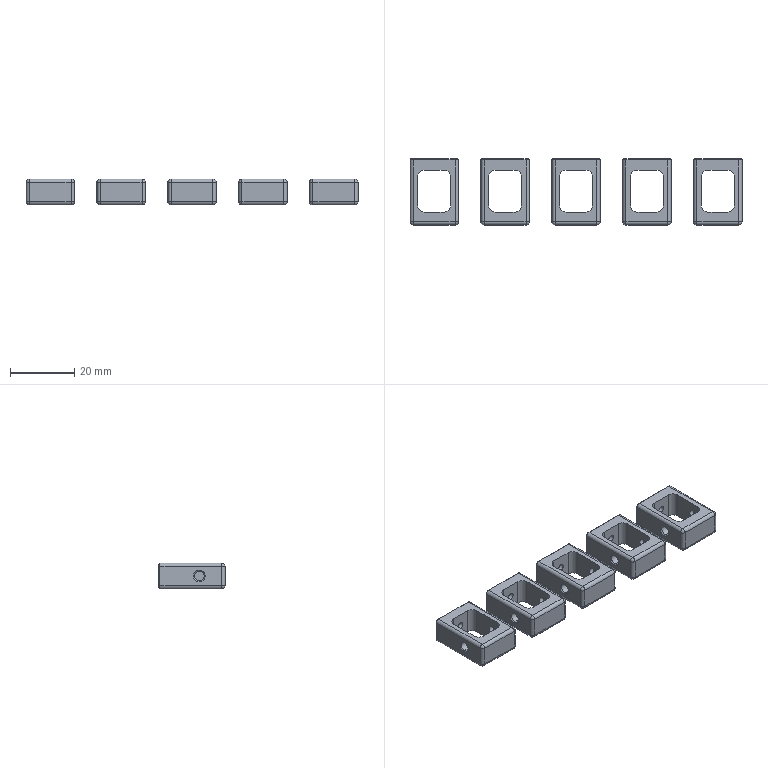NC program | NX | posted with a generic post | part box 103 x 20.5 x 8 mm
Lines 4727 to 5798 of 9732:
(ZLEVEL_PROFILE_COPY_1 , TOOL : D4)
N9440 T11 M6
N9442 G54
N9444 G17 G0 G90 X45.472 Y-3.85 S9950 M3
N9446 G43 Z30. H11
N9448 Z0.6
N9450 G94 G1 Z-0.4 F1000.
N9452 X45.587 Y-4.05
N9454 G3 X45.934 Y-4.25 R0.4
N9456 G1 X47.1 F1600.
N9458 Y-3.095
N9460 G3 X46.9 Y-2.749 R0.4
N9462 G1 X46.7 Y-2.634
N9464 Z0.6
N9466 G0 X45.472 Y-3.85 Z0.2
N9468 G1 Z-0.8 F1000.
N9470 X45.587 Y-4.05
N9472 G3 X45.934 Y-4.25 R0.4
N9474 G1 X47.1 F1600.
N9476 Y-3.095
N9478 G3 X46.9 Y-2.749 R0.4
N9480 G1 X46.7 Y-2.634
N9482 Z0.2
N9484 G0 X45.472 Y-3.85 Z-0.2
N9486 G1 Z-1.2 F1000.
N9488 X45.587 Y-4.05
N9490 G3 X45.934 Y-4.25 R0.4
N9492 G1 X47.1 F1600.
N9494 Y-3.095
N9496 G3 X46.9 Y-2.749 R0.4
N9498 G1 X46.7 Y-2.634
N9500 Z-0.2
N9502 G0 X45.472 Y-3.85 Z-0.6
N9504 G1 Z-1.6 F1000.
N9506 X45.587 Y-4.05
N9508 G3 X45.934 Y-4.25 R0.4
N9510 G1 X47.1 F1600.
N9512 Y-3.095
N9514 G3 X46.9 Y-2.749 R0.4
N9516 G1 X46.7 Y-2.634
N9518 Z-0.6
N9520 G0 X45.472 Y-3.85 Z-1.
N9522 G1 Z-2. F1000.
N9524 X45.587 Y-4.05
N9526 G3 X45.934 Y-4.25 R0.4
N9528 G1 X47.1 F1600.
N9530 Y-3.095
N9532 G3 X46.9 Y-2.749 R0.4
N9534 G1 X46.7 Y-2.634
N9536 Z-1.
N9538 G0 X45.472 Y-3.85 Z-1.4
N9540 G1 Z-2.4 F1000.
N9542 X45.587 Y-4.05
N9544 G3 X45.934 Y-4.25 R0.4
N9546 G1 X47.1 F1600.
N9548 Y-3.095
N9550 G3 X46.9 Y-2.749 R0.4
N9552 G1 X46.7 Y-2.634
N9554 Z-1.4
N9556 G0 X45.472 Y-3.85 Z-1.8
N9558 G1 Z-2.8 F1000.
N9560 X45.587 Y-4.05
N9562 G3 X45.934 Y-4.25 R0.4
N9564 G1 X47.1 F1600.
N9566 Y-3.095
N9568 G3 X46.9 Y-2.749 R0.4
N9570 G1 X46.7 Y-2.634
N9572 Z-1.8
N9574 G0 X45.472 Y-3.85 Z-2.2
N9576 G1 Z-3.2 F1000.
N9578 X45.587 Y-4.05
N9580 G3 X45.934 Y-4.25 R0.4
N9582 G1 X47.1 F1600.
N9584 Y-3.095
N9586 G3 X46.9 Y-2.749 R0.4
N9588 G1 X46.7 Y-2.634
N9590 Z-2.2
N9592 G0 X45.472 Y-3.85 Z-2.6
N9594 G1 Z-3.6 F1000.
N9596 X45.587 Y-4.05
N9598 G3 X45.934 Y-4.25 R0.4
N9600 G1 X47.1 F1600.
N9602 Y-3.095
N9604 G3 X46.9 Y-2.749 R0.4
N9606 G1 X46.7 Y-2.634
N9608 Z-2.6
N9610 G0 X45.472 Y-3.85 Z-3.
N9612 G1 Z-4. F1000.
N9614 X45.587 Y-4.05
N9616 G3 X45.934 Y-4.25 R0.4
N9618 G1 X47.1 F1600.
N9620 Y-3.095
N9622 G3 X46.9 Y-2.749 R0.4
N9624 G1 X46.7 Y-2.634
N9626 Z-3.
N9628 G0 X45.472 Y-3.85 Z-3.4
N9630 G1 Z-4.4 F1000.
N9632 X45.587 Y-4.05
N9634 G3 X45.934 Y-4.25 R0.4
N9636 G1 X47.1 F1600.
N9638 Y-3.095
N9640 G3 X46.9 Y-2.749 R0.4
N9642 G1 X46.7 Y-2.634
N9644 Z-3.4
N9646 G0 X45.472 Y-3.85 Z-3.8
N9648 G1 Z-4.8 F1000.
N9650 X45.587 Y-4.05
N9652 G3 X45.934 Y-4.25 R0.4
N9654 G1 X47.1 F1600.
N9656 Y-3.095
N9658 G3 X46.9 Y-2.749 R0.4
N9660 G1 X46.7 Y-2.634
N9662 Z-3.8
N9664 G0 X45.472 Y-3.85 Z-4.2
N9666 G1 Z-5.2 F1000.
N9668 X45.587 Y-4.05
N9670 G3 X45.934 Y-4.25 R0.4
N9672 G1 X47.1 F1600.
N9674 Y-3.095
N9676 G3 X46.9 Y-2.749 R0.4
N9678 G1 X46.7 Y-2.634
N9680 Z-4.2
N9682 G0 X45.472 Y-3.85 Z-4.6
N9684 G1 Z-5.6 F1000.
N9686 X45.587 Y-4.05
N9688 G3 X45.934 Y-4.25 R0.4
N9690 G1 X47.1 F1600.
N9692 Y-3.095
N9694 G3 X46.9 Y-2.749 R0.4
N9696 G1 X46.7 Y-2.634
N9698 Z-4.6
N9700 G0 X45.472 Y-3.85 Z-5.
N9702 G1 Z-6. F1000.
N9704 X45.587 Y-4.05
N9706 G3 X45.934 Y-4.25 R0.4
N9708 G1 X47.1 F1600.
N9710 Y-3.095
N9712 G3 X46.9 Y-2.749 R0.4
N9714 G1 X46.7 Y-2.634
N9716 Z-5.
N9718 G0 X45.472 Y-3.85 Z-5.4
N9720 G1 Z-6.4 F1000.
N9722 X45.587 Y-4.05
N9724 G3 X45.934 Y-4.25 R0.4
N9726 G1 X47.1 F1600.
N9728 Y-3.095
N9730 G3 X46.9 Y-2.749 R0.4
N9732 G1 X46.7 Y-2.634
N9734 Z-5.4
N9736 G0 X45.472 Y-3.85 Z-5.8
N9738 G1 Z-6.8 F1000.
N9740 X45.587 Y-4.05
N9742 G3 X45.934 Y-4.25 R0.4
N9744 G1 X47.1 F1600.
N9746 Y-3.095
N9748 G3 X46.9 Y-2.749 R0.4
N9750 G1 X46.7 Y-2.634
N9752 Z-5.8
N9754 G0 X45.472 Y-3.85 Z-6.2
N9756 G1 Z-7.2 F1000.
N9758 X45.587 Y-4.05
N9760 G3 X45.934 Y-4.25 R0.4
N9762 G1 X47.1 F1600.
N9764 Y-3.095
N9766 G3 X46.9 Y-2.749 R0.4
N9768 G1 X46.7 Y-2.634
N9770 Z-6.2
N9772 G0 X45.472 Y-3.85 Z-6.6
N9774 G1 Z-7.6 F1000.
N9776 X45.587 Y-4.05
N9778 G3 X45.934 Y-4.25 R0.4
N9780 G1 X47.1 F1600.
N9782 Y-3.095
N9784 G3 X46.9 Y-2.749 R0.4
N9786 G1 X46.7 Y-2.634
N9788 Z-6.6
N9790 G0 X45.472 Y-3.85 Z-7.
N9792 G1 Z-8. F1000.
N9794 X45.587 Y-4.05
N9796 G3 X45.934 Y-4.25 R0.4
N9798 G1 X47.1 F1600.
N9800 Y-3.095
N9802 G3 X46.9 Y-2.749 R0.4
N9804 G1 X46.7 Y-2.634
N9806 Z-7.
N9808 G0 Z30.
N9810 Y3.14
N9812 Z0.6
N9814 G1 Z-0.4 F1000.
N9816 X46.9 Y3.256
N9818 G3 X47.1 Y3.602 R0.4
N9820 G1 Y4.75 F1600.
N9822 X45.952
N9824 G3 X45.606 Y4.55 R0.4
N9826 G1 X45.49 Y4.35
N9828 Z0.6
N9830 G0 X46.7 Y3.14 Z0.2
N9832 G1 Z-0.8 F1000.
N9834 X46.9 Y3.256
N9836 G3 X47.1 Y3.602 R0.4
N9838 G1 Y4.75 F1600.
N9840 X45.952
N9842 G3 X45.606 Y4.55 R0.4
N9844 G1 X45.49 Y4.35
N9846 Z0.2
N9848 G0 X46.7 Y3.14 Z-0.2
N9850 G1 Z-1.2 F1000.
N9852 X46.9 Y3.256
N9854 G3 X47.1 Y3.602 R0.4
N9856 G1 Y4.75 F1600.
N9858 X45.952
N9860 G3 X45.606 Y4.55 R0.4
N9862 G1 X45.49 Y4.35
N9864 Z-0.2
N9866 G0 X46.7 Y3.14 Z-0.6
N9868 G1 Z-1.6 F1000.
N9870 X46.9 Y3.256
N9872 G3 X47.1 Y3.602 R0.4
N9874 G1 Y4.75 F1600.
N9876 X45.952
N9878 G3 X45.606 Y4.55 R0.4
N9880 G1 X45.49 Y4.35
N9882 Z-0.6
N9884 G0 X46.7 Y3.14 Z-1.
N9886 G1 Z-2. F1000.
N9888 X46.9 Y3.256
N9890 G3 X47.1 Y3.602 R0.4
N9892 G1 Y4.75 F1600.
N9894 X45.952
N9896 G3 X45.606 Y4.55 R0.4
N9898 G1 X45.49 Y4.35
N9900 Z-1.
N9902 G0 X46.7 Y3.14 Z-1.4
N9904 G1 Z-2.4 F1000.
N9906 X46.9 Y3.256
N9908 G3 X47.1 Y3.602 R0.4
N9910 G1 Y4.75 F1600.
N9912 X45.952
N9914 G3 X45.606 Y4.55 R0.4
N9916 G1 X45.49 Y4.35
N9918 Z-1.4
N9920 G0 X46.7 Y3.14 Z-1.8
N9922 G1 Z-2.8 F1000.
N9924 X46.9 Y3.256
N9926 G3 X47.1 Y3.602 R0.4
N9928 G1 Y4.75 F1600.
N9930 X45.952
N9932 G3 X45.606 Y4.55 R0.4
N9934 G1 X45.49 Y4.35
N9936 Z-1.8
N9938 G0 X46.7 Y3.14 Z-2.2
N9940 G1 Z-3.2 F1000.
N9942 X46.9 Y3.256
N9944 G3 X47.1 Y3.602 R0.4
N9946 G1 Y4.75 F1600.
N9948 X45.952
N9950 G3 X45.606 Y4.55 R0.4
N9952 G1 X45.49 Y4.35
N9954 Z-2.2
N9956 G0 X46.7 Y3.14 Z-2.6
N9958 G1 Z-3.6 F1000.
N9960 X46.9 Y3.256
N9962 G3 X47.1 Y3.602 R0.4
N9964 G1 Y4.75 F1600.
N9966 X45.952
N9968 G3 X45.606 Y4.55 R0.4
N9970 G1 X45.49 Y4.35
N9972 Z-2.6
N9974 G0 X46.7 Y3.14 Z-3.
N9976 G1 Z-4. F1000.
N9978 X46.9 Y3.256
N9980 G3 X47.1 Y3.602 R0.4
N9982 G1 Y4.75 F1600.
N9984 X45.952
N9986 G3 X45.606 Y4.55 R0.4
N9988 G1 X45.49 Y4.35
N9990 Z-3.
N9992 G0 X46.7 Y3.14 Z-3.4
N9994 G1 Z-4.4 F1000.
N9996 X46.9 Y3.256
N9998 G3 X47.1 Y3.602 R0.4
N10000 G1 Y4.75 F1600.
N10002 X45.952
N10004 G3 X45.606 Y4.55 R0.4
N10006 G1 X45.49 Y4.35
N10008 Z-3.4
N10010 G0 X46.7 Y3.14 Z-3.8
N10012 G1 Z-4.8 F1000.
N10014 X46.9 Y3.256
N10016 G3 X47.1 Y3.602 R0.4
N10018 G1 Y4.75 F1600.
N10020 X45.952
N10022 G3 X45.606 Y4.55 R0.4
N10024 G1 X45.49 Y4.35
N10026 Z-3.8
N10028 G0 X46.7 Y3.14 Z-4.2
N10030 G1 Z-5.2 F1000.
N10032 X46.9 Y3.256
N10034 G3 X47.1 Y3.602 R0.4
N10036 G1 Y4.75 F1600.
N10038 X45.952
N10040 G3 X45.606 Y4.55 R0.4
N10042 G1 X45.49 Y4.35
N10044 Z-4.2
N10046 G0 X46.7 Y3.14 Z-4.6
N10048 G1 Z-5.6 F1000.
N10050 X46.9 Y3.256
N10052 G3 X47.1 Y3.602 R0.4
N10054 G1 Y4.75 F1600.
N10056 X45.952
N10058 G3 X45.606 Y4.55 R0.4
N10060 G1 X45.49 Y4.35
N10062 Z-4.6
N10064 G0 X46.7 Y3.14 Z-5.
N10066 G1 Z-6. F1000.
N10068 X46.9 Y3.256
N10070 G3 X47.1 Y3.602 R0.4
N10072 G1 Y4.75 F1600.
N10074 X45.952
N10076 G3 X45.606 Y4.55 R0.4
N10078 G1 X45.49 Y4.35
N10080 Z-5.
N10082 G0 X46.7 Y3.14 Z-5.4
N10084 G1 Z-6.4 F1000.
N10086 X46.9 Y3.256
N10088 G3 X47.1 Y3.602 R0.4
N10090 G1 Y4.75 F1600.
N10092 X45.952
N10094 G3 X45.606 Y4.55 R0.4
N10096 G1 X45.49 Y4.35
N10098 Z-5.4
N10100 G0 X46.7 Y3.14 Z-5.8
N10102 G1 Z-6.8 F1000.
N10104 X46.9 Y3.256
N10106 G3 X47.1 Y3.602 R0.4
N10108 G1 Y4.75 F1600.
N10110 X45.952
N10112 G3 X45.606 Y4.55 R0.4
N10114 G1 X45.49 Y4.35
N10116 Z-5.8
N10118 G0 X46.7 Y3.14 Z-6.2
N10120 G1 Z-7.2 F1000.
N10122 X46.9 Y3.256
N10124 G3 X47.1 Y3.602 R0.4
N10126 G1 Y4.75 F1600.
N10128 X45.952
N10130 G3 X45.606 Y4.55 R0.4
N10132 G1 X45.49 Y4.35
N10134 Z-6.2
N10136 G0 X46.7 Y3.14 Z-6.6
N10138 G1 Z-7.6 F1000.
N10140 X46.9 Y3.256
N10142 G3 X47.1 Y3.602 R0.4
N10144 G1 Y4.75 F1600.
N10146 X45.952
N10148 G3 X45.606 Y4.55 R0.4
N10150 G1 X45.49 Y4.35
N10152 Z-6.6
N10154 G0 X46.7 Y3.14 Z-7.
N10156 G1 Z-8. F1000.
N10158 X46.9 Y3.256
N10160 G3 X47.1 Y3.602 R0.4
N10162 G1 Y4.75 F1600.
N10164 X45.952
N10166 G3 X45.606 Y4.55 R0.4
N10168 G1 X45.49 Y4.35
N10170 Z-7.
N10172 G0 Z30.
N10174 X42.535
N10176 Z0.6
N10178 G1 Z-0.4 F1000.
N10180 X42.419 Y4.55
N10182 G3 X42.073 Y4.75 R0.4
N10184 G1 X40.9 F1600.
N10186 Y3.522
N10188 G3 X41.1 Y3.175 R0.4
N10190 G1 X41.3 Y3.06
N10192 Z0.6
N10194 G0 X42.535 Y4.35 Z0.2
N10196 G1 Z-0.8 F1000.
N10198 X42.419 Y4.55
N10200 G3 X42.073 Y4.75 R0.4
N10202 G1 X40.9 F1600.
N10204 Y3.522
N10206 G3 X41.1 Y3.175 R0.4
N10208 G1 X41.3 Y3.06
N10210 Z0.2
N10212 G0 X42.535 Y4.35 Z-0.2
N10214 G1 Z-1.2 F1000.
N10216 X42.419 Y4.55
N10218 G3 X42.073 Y4.75 R0.4
N10220 G1 X40.9 F1600.
N10222 Y3.522
N10224 G3 X41.1 Y3.175 R0.4
N10226 G1 X41.3 Y3.06
N10228 Z-0.2
N10230 G0 X42.535 Y4.35 Z-0.6
N10232 G1 Z-1.6 F1000.
N10234 X42.419 Y4.55
N10236 G3 X42.073 Y4.75 R0.4
N10238 G1 X40.9 F1600.
N10240 Y3.522
N10242 G3 X41.1 Y3.175 R0.4
N10244 G1 X41.3 Y3.06
N10246 Z-0.6
N10248 G0 X42.535 Y4.35 Z-1.
N10250 G1 Z-2. F1000.
N10252 X42.419 Y4.55
N10254 G3 X42.073 Y4.75 R0.4
N10256 G1 X40.9 F1600.
N10258 Y3.522
N10260 G3 X41.1 Y3.175 R0.4
N10262 G1 X41.3 Y3.06
N10264 Z-1.
N10266 G0 X42.535 Y4.35 Z-1.4
N10268 G1 Z-2.4 F1000.
N10270 X42.419 Y4.55
N10272 G3 X42.073 Y4.75 R0.4
N10274 G1 X40.9 F1600.
N10276 Y3.522
N10278 G3 X41.1 Y3.175 R0.4
N10280 G1 X41.3 Y3.06
N10282 Z-1.4
N10284 G0 X42.535 Y4.35 Z-1.8
N10286 G1 Z-2.8 F1000.
N10288 X42.419 Y4.55
N10290 G3 X42.073 Y4.75 R0.4
N10292 G1 X40.9 F1600.
N10294 Y3.522
N10296 G3 X41.1 Y3.175 R0.4
N10298 G1 X41.3 Y3.06
N10300 Z-1.8
N10302 G0 X42.535 Y4.35 Z-2.2
N10304 G1 Z-3.2 F1000.
N10306 X42.419 Y4.55
N10308 G3 X42.073 Y4.75 R0.4
N10310 G1 X40.9 F1600.
N10312 Y3.522
N10314 G3 X41.1 Y3.175 R0.4
N10316 G1 X41.3 Y3.06
N10318 Z-2.2
N10320 G0 X42.535 Y4.35 Z-2.6
N10322 G1 Z-3.6 F1000.
N10324 X42.419 Y4.55
N10326 G3 X42.073 Y4.75 R0.4
N10328 G1 X40.9 F1600.
N10330 Y3.522
N10332 G3 X41.1 Y3.175 R0.4
N10334 G1 X41.3 Y3.06
N10336 Z-2.6
N10338 G0 X42.535 Y4.35 Z-3.
N10340 G1 Z-4. F1000.
N10342 X42.419 Y4.55
N10344 G3 X42.073 Y4.75 R0.4
N10346 G1 X40.9 F1600.
N10348 Y3.522
N10350 G3 X41.1 Y3.175 R0.4
N10352 G1 X41.3 Y3.06
N10354 Z-3.
N10356 G0 X42.535 Y4.35 Z-3.4
N10358 G1 Z-4.4 F1000.
N10360 X42.419 Y4.55
N10362 G3 X42.073 Y4.75 R0.4
N10364 G1 X40.9 F1600.
N10366 Y3.522
N10368 G3 X41.1 Y3.175 R0.4
N10370 G1 X41.3 Y3.06
N10372 Z-3.4
N10374 G0 X42.535 Y4.35 Z-3.8
N10376 G1 Z-4.8 F1000.
N10378 X42.419 Y4.55
N10380 G3 X42.073 Y4.75 R0.4
N10382 G1 X40.9 F1600.
N10384 Y3.522
N10386 G3 X41.1 Y3.175 R0.4
N10388 G1 X41.3 Y3.06
N10390 Z-3.8
N10392 G0 X42.535 Y4.35 Z-4.2
N10394 G1 Z-5.2 F1000.
N10396 X42.419 Y4.55
N10398 G3 X42.073 Y4.75 R0.4
N10400 G1 X40.9 F1600.
N10402 Y3.522
N10404 G3 X41.1 Y3.175 R0.4
N10406 G1 X41.3 Y3.06
N10408 Z-4.2
N10410 G0 X42.535 Y4.35 Z-4.6
N10412 G1 Z-5.6 F1000.
N10414 X42.419 Y4.55
N10416 G3 X42.073 Y4.75 R0.4
N10418 G1 X40.9 F1600.
N10420 Y3.522
N10422 G3 X41.1 Y3.175 R0.4
N10424 G1 X41.3 Y3.06
N10426 Z-4.6
N10428 G0 X42.535 Y4.35 Z-5.
N10430 G1 Z-6. F1000.
N10432 X42.419 Y4.55
N10434 G3 X42.073 Y4.75 R0.4
N10436 G1 X40.9 F1600.
N10438 Y3.522
N10440 G3 X41.1 Y3.175 R0.4
N10442 G1 X41.3 Y3.06
N10444 Z-5.
N10446 G0 X42.535 Y4.35 Z-5.4
N10448 G1 Z-6.4 F1000.
N10450 X42.419 Y4.55
N10452 G3 X42.073 Y4.75 R0.4
N10454 G1 X40.9 F1600.
N10456 Y3.522
N10458 G3 X41.1 Y3.175 R0.4
N10460 G1 X41.3 Y3.06
N10462 Z-5.4
N10464 G0 X42.535 Y4.35 Z-5.8
N10466 G1 Z-6.8 F1000.
N10468 X42.419 Y4.55
N10470 G3 X42.073 Y4.75 R0.4
N10472 G1 X40.9 F1600.
N10474 Y3.522
N10476 G3 X41.1 Y3.175 R0.4
N10478 G1 X41.3 Y3.06
N10480 Z-5.8
N10482 G0 X42.535 Y4.35 Z-6.2
N10484 G1 Z-7.2 F1000.
N10486 X42.419 Y4.55
N10488 G3 X42.073 Y4.75 R0.4
N10490 G1 X40.9 F1600.
N10492 Y3.522
N10494 G3 X41.1 Y3.175 R0.4
N10496 G1 X41.3 Y3.06
N10498 Z-6.2
N10500 G0 X42.535 Y4.35 Z-6.6
N10502 G1 Z-7.6 F1000.
N10504 X42.419 Y4.55
N10506 G3 X42.073 Y4.75 R0.4
N10508 G1 X40.9 F1600.
N10510 Y3.522
N10512 G3 X41.1 Y3.175 R0.4
N10514 G1 X41.3 Y3.06
N10516 Z-6.6
N10518 G0 X42.535 Y4.35 Z-7.
N10520 G1 Z-8. F1000.
N10522 X42.419 Y4.55
N10524 G3 X42.073 Y4.75 R0.4
N10526 G1 X40.9 F1600.
N10528 Y3.522
N10530 G3 X41.1 Y3.175 R0.4
N10532 G1 X41.3 Y3.06
N10534 Z-7.
N10536 G0 Z30.
N10538 Y-2.634
N10540 Z0.6
N10542 G1 Z-0.4 F1000.
N10544 X41.1 Y-2.749
N10546 G3 X40.9 Y-3.095 R0.4
N10548 G1 Y-4.25 F1600.
N10550 X42.066
N10552 G3 X42.413 Y-4.05 R0.4
N10554 G1 X42.528 Y-3.85
N10556 Z0.6
N10558 G0 X41.3 Y-2.634 Z0.2
N10560 G1 Z-0.8 F1000.
N10562 X41.1 Y-2.749
N10564 G3 X40.9 Y-3.095 R0.4
N10566 G1 Y-4.25 F1600.
N10568 X42.066
N10570 G3 X42.413 Y-4.05 R0.4
N10572 G1 X42.528 Y-3.85
N10574 Z0.2
N10576 G0 X41.3 Y-2.634 Z-0.2
N10578 G1 Z-1.2 F1000.
N10580 X41.1 Y-2.749
N10582 G3 X40.9 Y-3.095 R0.4
N10584 G1 Y-4.25 F1600.
N10586 X42.066
N10588 G3 X42.413 Y-4.05 R0.4
N10590 G1 X42.528 Y-3.85
N10592 Z-0.2
N10594 G0 X41.3 Y-2.634 Z-0.6
N10596 G1 Z-1.6 F1000.
N10598 X41.1 Y-2.749
N10600 G3 X40.9 Y-3.095 R0.4
N10602 G1 Y-4.25 F1600.
N10604 X42.066
N10606 G3 X42.413 Y-4.05 R0.4
N10608 G1 X42.528 Y-3.85
N10610 Z-0.6
N10612 G0 X41.3 Y-2.634 Z-1.
N10614 G1 Z-2. F1000.
N10616 X41.1 Y-2.749
N10618 G3 X40.9 Y-3.095 R0.4
N10620 G1 Y-4.25 F1600.
N10622 X42.066
N10624 G3 X42.413 Y-4.05 R0.4
N10626 G1 X42.528 Y-3.85
N10628 Z-1.
N10630 G0 X41.3 Y-2.634 Z-1.4
N10632 G1 Z-2.4 F1000.
N10634 X41.1 Y-2.749
N10636 G3 X40.9 Y-3.095 R0.4
N10638 G1 Y-4.25 F1600.
N10640 X42.066
N10642 G3 X42.413 Y-4.05 R0.4
N10644 G1 X42.528 Y-3.85
N10646 Z-1.4
N10648 G0 X41.3 Y-2.634 Z-1.8
N10650 G1 Z-2.8 F1000.
N10652 X41.1 Y-2.749
N10654 G3 X40.9 Y-3.095 R0.4
N10656 G1 Y-4.25 F1600.
N10658 X42.066
N10660 G3 X42.413 Y-4.05 R0.4
N10662 G1 X42.528 Y-3.85
N10664 Z-1.8
N10666 G0 X41.3 Y-2.634 Z-2.2
N10668 G1 Z-3.2 F1000.
N10670 X41.1 Y-2.749
N10672 G3 X40.9 Y-3.095 R0.4
N10674 G1 Y-4.25 F1600.
N10676 X42.066
N10678 G3 X42.413 Y-4.05 R0.4
N10680 G1 X42.528 Y-3.85
N10682 Z-2.2
N10684 G0 X41.3 Y-2.634 Z-2.6
N10686 G1 Z-3.6 F1000.
N10688 X41.1 Y-2.749
N10690 G3 X40.9 Y-3.095 R0.4
N10692 G1 Y-4.25 F1600.
N10694 X42.066
N10696 G3 X42.413 Y-4.05 R0.4
N10698 G1 X42.528 Y-3.85
N10700 Z-2.6
N10702 G0 X41.3 Y-2.634 Z-3.
N10704 G1 Z-4. F1000.
N10706 X41.1 Y-2.749
N10708 G3 X40.9 Y-3.095 R0.4
N10710 G1 Y-4.25 F1600.
N10712 X42.066
N10714 G3 X42.413 Y-4.05 R0.4
N10716 G1 X42.528 Y-3.85
N10718 Z-3.
N10720 G0 X41.3 Y-2.634 Z-3.4
N10722 G1 Z-4.4 F1000.
N10724 X41.1 Y-2.749
N10726 G3 X40.9 Y-3.095 R0.4
N10728 G1 Y-4.25 F1600.
N10730 X42.066
N10732 G3 X42.413 Y-4.05 R0.4
N10734 G1 X42.528 Y-3.85
N10736 Z-3.4
N10738 G0 X41.3 Y-2.634 Z-3.8
N10740 G1 Z-4.8 F1000.
N10742 X41.1 Y-2.749
N10744 G3 X40.9 Y-3.095 R0.4
N10746 G1 Y-4.25 F1600.
N10748 X42.066
N10750 G3 X42.413 Y-4.05 R0.4
N10752 G1 X42.528 Y-3.85
N10754 Z-3.8
N10756 G0 X41.3 Y-2.634 Z-4.2
N10758 G1 Z-5.2 F1000.
N10760 X41.1 Y-2.749
N10762 G3 X40.9 Y-3.095 R0.4
N10764 G1 Y-4.25 F1600.
N10766 X42.066
N10768 G3 X42.413 Y-4.05 R0.4
N10770 G1 X42.528 Y-3.85
N10772 Z-4.2
N10774 G0 X41.3 Y-2.634 Z-4.6
N10776 G1 Z-5.6 F1000.
N10778 X41.1 Y-2.749
N10780 G3 X40.9 Y-3.095 R0.4
N10782 G1 Y-4.25 F1600.
N10784 X42.066
N10786 G3 X42.413 Y-4.05 R0.4
N10788 G1 X42.528 Y-3.85
N10790 Z-4.6
N10792 G0 X41.3 Y-2.634 Z-5.
N10794 G1 Z-6. F1000.
N10796 X41.1 Y-2.749
N10798 G3 X40.9 Y-3.095 R0.4
N10800 G1 Y-4.25 F1600.
N10802 X42.066
N10804 G3 X42.413 Y-4.05 R0.4
N10806 G1 X42.528 Y-3.85
N10808 Z-5.
N10810 G0 X41.3 Y-2.634 Z-5.4
N10812 G1 Z-6.4 F1000.
N10814 X41.1 Y-2.749
N10816 G3 X40.9 Y-3.095 R0.4
N10818 G1 Y-4.25 F1600.
N10820 X42.066
N10822 G3 X42.413 Y-4.05 R0.4
N10824 G1 X42.528 Y-3.85
N10826 Z-5.4
N10828 G0 X41.3 Y-2.634 Z-5.8
N10830 G1 Z-6.8 F1000.
N10832 X41.1 Y-2.749
N10834 G3 X40.9 Y-3.095 R0.4
N10836 G1 Y-4.25 F1600.
N10838 X42.066
N10840 G3 X42.413 Y-4.05 R0.4
N10842 G1 X42.528 Y-3.85
N10844 Z-5.8
N10846 G0 X41.3 Y-2.634 Z-6.2
N10848 G1 Z-7.2 F1000.
N10850 X41.1 Y-2.749
N10852 G3 X40.9 Y-3.095 R0.4
N10854 G1 Y-4.25 F1600.
N10856 X42.066
N10858 G3 X42.413 Y-4.05 R0.4
N10860 G1 X42.528 Y-3.85
N10862 Z-6.2
N10864 G0 X41.3 Y-2.634 Z-6.6
N10866 G1 Z-7.6 F1000.
N10868 X41.1 Y-2.749
N10870 G3 X40.9 Y-3.095 R0.4
N10872 G1 Y-4.25 F1600.
N10874 X42.066
N10876 G3 X42.413 Y-4.05 R0.4
N10878 G1 X42.528 Y-3.85
N10880 Z-6.6
N10882 G0 X41.3 Y-2.634 Z-7.
N10884 G1 Z-8. F1000.
N10886 X41.1 Y-2.749
N10888 G3 X40.9 Y-3.095 R0.4
N10890 G1 Y-4.25 F1600.
N10892 X42.066
N10894 G3 X42.413 Y-4.05 R0.4
N10896 G1 X42.528 Y-3.85
N10898 Z-7.
N10900 G0 Z53.
N10902 X23.472
N10904 Z0.6
N10906 G1 Z-0.4 F1000.
N10908 X23.587 Y-4.05
N10910 G3 X23.934 Y-4.25 R0.4
N10912 G1 X25.1 F1600.
N10914 Y-3.096
N10916 G3 X24.9 Y-2.75 R0.4
N10918 G1 X24.7 Y-2.635
N10920 Z0.6
N10922 G0 X23.472 Y-3.85 Z0.2
N10924 G1 Z-0.8 F1000.
N10926 X23.587 Y-4.05
N10928 G3 X23.934 Y-4.25 R0.4
N10930 G1 X25.1 F1600.
N10932 Y-3.096
N10934 G3 X24.9 Y-2.75 R0.4
N10936 G1 X24.7 Y-2.635
N10938 Z0.2
N10940 G0 X23.472 Y-3.85 Z-0.2
N10942 G1 Z-1.2 F1000.
N10944 X23.587 Y-4.05
N10946 G3 X23.934 Y-4.25 R0.4
N10948 G1 X25.1 F1600.
N10950 Y-3.096
N10952 G3 X24.9 Y-2.75 R0.4
N10954 G1 X24.7 Y-2.635
N10956 Z-0.2
N10958 G0 X23.472 Y-3.85 Z-0.6
N10960 G1 Z-1.6 F1000.
N10962 X23.587 Y-4.05
N10964 G3 X23.934 Y-4.25 R0.4
N10966 G1 X25.1 F1600.
N10968 Y-3.096
N10970 G3 X24.9 Y-2.75 R0.4
N10972 G1 X24.7 Y-2.635
N10974 Z-0.6
N10976 G0 X23.472 Y-3.85 Z-1.
N10978 G1 Z-2. F1000.
N10980 X23.587 Y-4.05
N10982 G3 X23.934 Y-4.25 R0.4
N10984 G1 X25.1 F1600.
N10986 Y-3.096
N10988 G3 X24.9 Y-2.75 R0.4
N10990 G1 X24.7 Y-2.635
N10992 Z-1.
N10994 G0 X23.472 Y-3.85 Z-1.4
N10996 G1 Z-2.4 F1000.
N10998 X23.587 Y-4.05
N11000 G3 X23.934 Y-4.25 R0.4
N11002 G1 X25.1 F1600.
N11004 Y-3.096
N11006 G3 X24.9 Y-2.75 R0.4
N11008 G1 X24.7 Y-2.635
N11010 Z-1.4
N11012 G0 X23.472 Y-3.85 Z-1.8
N11014 G1 Z-2.8 F1000.
N11016 X23.587 Y-4.05
N11018 G3 X23.934 Y-4.25 R0.4
N11020 G1 X25.1 F1600.
N11022 Y-3.096
N11024 G3 X24.9 Y-2.75 R0.4
N11026 G1 X24.7 Y-2.635
N11028 Z-1.8
N11030 G0 X23.472 Y-3.85 Z-2.2
N11032 G1 Z-3.2 F1000.
N11034 X23.587 Y-4.05
N11036 G3 X23.934 Y-4.25 R0.4
N11038 G1 X25.1 F1600.
N11040 Y-3.096
N11042 G3 X24.9 Y-2.75 R0.4
N11044 G1 X24.7 Y-2.635
N11046 Z-2.2
N11048 G0 X23.472 Y-3.85 Z-2.6
N11050 G1 Z-3.6 F1000.
N11052 X23.587 Y-4.05
N11054 G3 X23.934 Y-4.25 R0.4
N11056 G1 X25.1 F1600.
N11058 Y-3.096
N11060 G3 X24.9 Y-2.75 R0.4
N11062 G1 X24.7 Y-2.635
N11064 Z-2.6
N11066 G0 X23.472 Y-3.85 Z-3.
N11068 G1 Z-4. F1000.
N11070 X23.587 Y-4.05
N11072 G3 X23.934 Y-4.25 R0.4
N11074 G1 X25.1 F1600.
N11076 Y-3.096
N11078 G3 X24.9 Y-2.75 R0.4
N11080 G1 X24.7 Y-2.635
N11082 Z-3.
N11084 G0 X23.472 Y-3.85 Z-3.4
N11086 G1 Z-4.4 F1000.
N11088 X23.587 Y-4.05
N11090 G3 X23.934 Y-4.25 R0.4
N11092 G1 X25.1 F1600.
N11094 Y-3.096
N11096 G3 X24.9 Y-2.75 R0.4
N11098 G1 X24.7 Y-2.635
N11100 Z-3.4
N11102 G0 X23.472 Y-3.85 Z-3.8
N11104 G1 Z-4.8 F1000.
N11106 X23.587 Y-4.05
N11108 G3 X23.934 Y-4.25 R0.4
N11110 G1 X25.1 F1600.
N11112 Y-3.096
N11114 G3 X24.9 Y-2.75 R0.4
N11116 G1 X24.7 Y-2.635
N11118 Z-3.8
N11120 G0 X23.472 Y-3.85 Z-4.2
N11122 G1 Z-5.2 F1000.
N11124 X23.587 Y-4.05
N11126 G3 X23.934 Y-4.25 R0.4
N11128 G1 X25.1 F1600.
N11130 Y-3.096
N11132 G3 X24.9 Y-2.75 R0.4
N11134 G1 X24.7 Y-2.635
N11136 Z-4.2
N11138 G0 X23.472 Y-3.85 Z-4.6
N11140 G1 Z-5.6 F1000.
N11142 X23.587 Y-4.05
N11144 G3 X23.934 Y-4.25 R0.4
N11146 G1 X25.1 F1600.
N11148 Y-3.096
N11150 G3 X24.9 Y-2.75 R0.4
N11152 G1 X24.7 Y-2.635
N11154 Z-4.6
N11156 G0 X23.472 Y-3.85 Z-5.
N11158 G1 Z-6. F1000.
N11160 X23.587 Y-4.05
N11162 G3 X23.934 Y-4.25 R0.4
N11164 G1 X25.1 F1600.
N11166 Y-3.096
N11168 G3 X24.9 Y-2.75 R0.4
N11170 G1 X24.7 Y-2.635
N11172 Z-5.
N11174 G0 X23.472 Y-3.85 Z-5.4
N11176 G1 Z-6.4 F1000.
N11178 X23.587 Y-4.05
N11180 G3 X23.934 Y-4.25 R0.4
N11182 G1 X25.1 F1600.
N11184 Y-3.096
N11186 G3 X24.9 Y-2.75 R0.4
N11188 G1 X24.7 Y-2.635
N11190 Z-5.4
N11192 G0 X23.472 Y-3.85 Z-5.8
N11194 G1 Z-6.8 F1000.
N11196 X23.587 Y-4.05
N11198 G3 X23.934 Y-4.25 R0.4
N11200 G1 X25.1 F1600.
N11202 Y-3.096
N11204 G3 X24.9 Y-2.75 R0.4
N11206 G1 X24.7 Y-2.635
N11208 Z-5.8
N11210 G0 X23.472 Y-3.85 Z-6.2
N11212 G1 Z-7.2 F1000.
N11214 X23.587 Y-4.05
N11216 G3 X23.934 Y-4.25 R0.4
N11218 G1 X25.1 F1600.
N11220 Y-3.096
N11222 G3 X24.9 Y-2.75 R0.4
N11224 G1 X24.7 Y-2.635
N11226 Z-6.2
N11228 G0 X23.472 Y-3.85 Z-6.6
N11230 G1 Z-7.6 F1000.
N11232 X23.587 Y-4.05
N11234 G3 X23.934 Y-4.25 R0.4
N11236 G1 X25.1 F1600.
N11238 Y-3.096
N11240 G3 X24.9 Y-2.75 R0.4
N11242 G1 X24.7 Y-2.635
N11244 Z-6.6
N11246 G0 X23.472 Y-3.85 Z-7.
N11248 G1 Z-8. F1000.
N11250 X23.587 Y-4.05
N11252 G3 X23.934 Y-4.25 R0.4
N11254 G1 X25.1 F1600.
N11256 Y-3.096
N11258 G3 X24.9 Y-2.75 R0.4
N11260 G1 X24.7 Y-2.635
N11262 Z-7.
N11264 G0 Z30.
N11266 Y3.139
N11268 Z0.6
N11270 G1 Z-0.4 F1000.
N11272 X24.9 Y3.255
N11274 G3 X25.1 Y3.601 R0.4
N11276 G1 Y4.75 F1600.
N11278 X23.95
N11280 G3 X23.604 Y4.55 R0.4
N11282 G1 X23.489 Y4.35
N11284 Z0.6
N11286 G0 X24.7 Y3.139 Z0.2
N11288 G1 Z-0.8 F1000.
N11290 X24.9 Y3.255
N11292 G3 X25.1 Y3.601 R0.4
N11294 G1 Y4.75 F1600.
N11296 X23.95
N11298 G3 X23.604 Y4.55 R0.4
N11300 G1 X23.489 Y4.35
N11302 Z0.2
N11304 G0 X24.7 Y3.139 Z-0.2
N11306 G1 Z-1.2 F1000.
N11308 X24.9 Y3.255
N11310 G3 X25.1 Y3.601 R0.4
N11312 G1 Y4.75 F1600.
N11314 X23.95
N11316 G3 X23.604 Y4.55 R0.4
N11318 G1 X23.489 Y4.35
N11320 Z-0.2
N11322 G0 X24.7 Y3.139 Z-0.6
N11324 G1 Z-1.6 F1000.
N11326 X24.9 Y3.255
N11328 G3 X25.1 Y3.601 R0.4
N11330 G1 Y4.75 F1600.
N11332 X23.95
N11334 G3 X23.604 Y4.55 R0.4
N11336 G1 X23.489 Y4.35
N11338 Z-0.6
N11340 G0 X24.7 Y3.139 Z-1.
N11342 G1 Z-2. F1000.
N11344 X24.9 Y3.255
N11346 G3 X25.1 Y3.601 R0.4
N11348 G1 Y4.75 F1600.
N11350 X23.95
N11352 G3 X23.604 Y4.55 R0.4
N11354 G1 X23.489 Y4.35
N11356 Z-1.
N11358 G0 X24.7 Y3.139 Z-1.4
N11360 G1 Z-2.4 F1000.
N11362 X24.9 Y3.255
N11364 G3 X25.1 Y3.601 R0.4
N11366 G1 Y4.75 F1600.
N11368 X23.95
N11370 G3 X23.604 Y4.55 R0.4
N11372 G1 X23.489 Y4.35
N11374 Z-1.4
N11376 G0 X24.7 Y3.139 Z-1.8
N11378 G1 Z-2.8 F1000.
N11380 X24.9 Y3.255
N11382 G3 X25.1 Y3.601 R0.4
N11384 G1 Y4.75 F1600.
N11386 X23.95
N11388 G3 X23.604 Y4.55 R0.4
N11390 G1 X23.489 Y4.35
N11392 Z-1.8
N11394 G0 X24.7 Y3.139 Z-2.2
N11396 G1 Z-3.2 F1000.
N11398 X24.9 Y3.255
N11400 G3 X25.1 Y3.601 R0.4
N11402 G1 Y4.75 F1600.
N11404 X23.95
N11406 G3 X23.604 Y4.55 R0.4
N11408 G1 X23.489 Y4.35
N11410 Z-2.2
N11412 G0 X24.7 Y3.139 Z-2.6
N11414 G1 Z-3.6 F1000.
N11416 X24.9 Y3.255
N11418 G3 X25.1 Y3.601 R0.4
N11420 G1 Y4.75 F1600.
N11422 X23.95
N11424 G3 X23.604 Y4.55 R0.4
N11426 G1 X23.489 Y4.35
N11428 Z-2.6
N11430 G0 X24.7 Y3.139 Z-3.
N11432 G1 Z-4. F1000.
N11434 X24.9 Y3.255
N11436 G3 X25.1 Y3.601 R0.4
N11438 G1 Y4.75 F1600.
N11440 X23.95
N11442 G3 X23.604 Y4.55 R0.4
N11444 G1 X23.489 Y4.35
N11446 Z-3.
N11448 G0 X24.7 Y3.139 Z-3.4
N11450 G1 Z-4.4 F1000.
N11452 X24.9 Y3.255
N11454 G3 X25.1 Y3.601 R0.4
N11456 G1 Y4.75 F1600.
N11458 X23.95
N11460 G3 X23.604 Y4.55 R0.4
N11462 G1 X23.489 Y4.35
N11464 Z-3.4
N11466 G0 X24.7 Y3.139 Z-3.8
N11468 G1 Z-4.8 F1000.
N11470 X24.9 Y3.255
N11472 G3 X25.1 Y3.601 R0.4
N11474 G1 Y4.75 F1600.
N11476 X23.95
N11478 G3 X23.604 Y4.55 R0.4
N11480 G1 X23.489 Y4.35
N11482 Z-3.8
N11484 G0 X24.7 Y3.139 Z-4.2
N11486 G1 Z-5.2 F1000.
N11488 X24.9 Y3.255
N11490 G3 X25.1 Y3.601 R0.4
N11492 G1 Y4.75 F1600.
N11494 X23.95
N11496 G3 X23.604 Y4.55 R0.4
N11498 G1 X23.489 Y4.35
N11500 Z-4.2
N11502 G0 X24.7 Y3.139 Z-4.6
N11504 G1 Z-5.6 F1000.
N11506 X24.9 Y3.255
N11508 G3 X25.1 Y3.601 R0.4
N11510 G1 Y4.75 F1600.
N11512 X23.95
N11514 G3 X23.604 Y4.55 R0.4
N11516 G1 X23.489 Y4.35
N11518 Z-4.6
N11520 G0 X24.7 Y3.139 Z-5.
N11522 G1 Z-6. F1000.
N11524 X24.9 Y3.255
N11526 G3 X25.1 Y3.601 R0.4
N11528 G1 Y4.75 F1600.
N11530 X23.95
N11532 G3 X23.604 Y4.55 R0.4
N11534 G1 X23.489 Y4.35
N11536 Z-5.
N11538 G0 X24.7 Y3.139 Z-5.4
N11540 G1 Z-6.4 F1000.
N11542 X24.9 Y3.255
N11544 G3 X25.1 Y3.601 R0.4
N11546 G1 Y4.75 F1600.
N11548 X23.95
N11550 G3 X23.604 Y4.55 R0.4
N11552 G1 X23.489 Y4.35
N11554 Z-5.4
N11556 G0 X24.7 Y3.139 Z-5.8
N11558 G1 Z-6.8 F1000.
N11560 X24.9 Y3.255
N11562 G3 X25.1 Y3.601 R0.4
N11564 G1 Y4.75 F1600.
N11566 X23.95
N11568 G3 X23.604 Y4.55 R0.4
N11570 G1 X23.489 Y4.35
N11572 Z-5.8
N11574 G0 X24.7 Y3.139 Z-6.2
N11576 G1 Z-7.2 F1000.